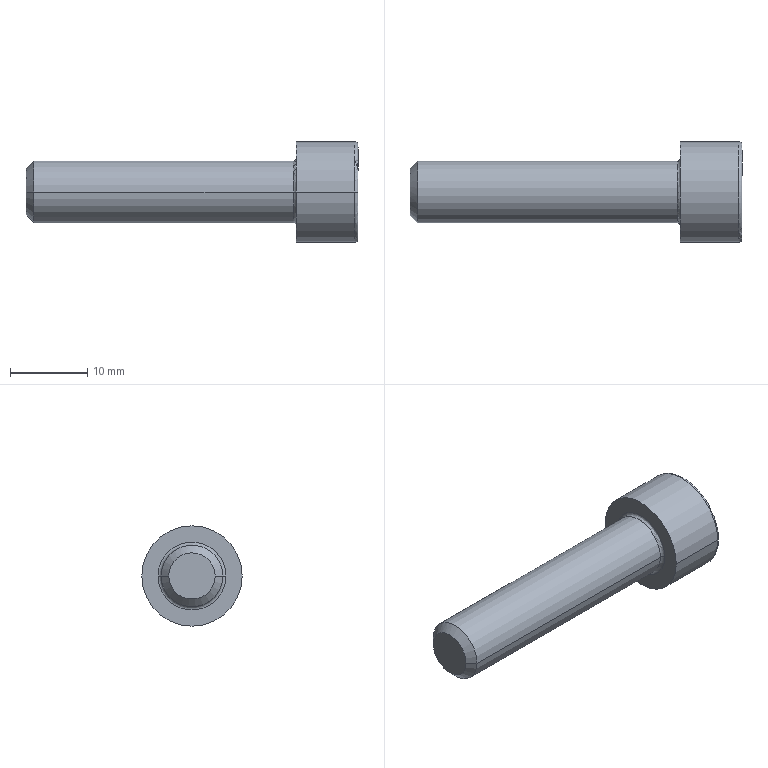Part | STEP file | Positioning_id2042_x_t | 1 solid | 20 faces | box 43 x 13 x 13 mm | volume 2687 mm3 | plane 10 | torus 4 | cylinder 4 | cone 2 | commonest cylinder face diameters 8 x2 13 x2
STEP:
#1=CARTESIAN_POINT('',(0.,0.,0.));
#2=DIRECTION('',(0.,0.,1.));
#3=DIRECTION('',(1.,0.,0.));
#4=AXIS2_PLACEMENT_3D('',#1,#2,#3);
#5=CARTESIAN_POINT('',(-1027.002,-38.,396.5));
#6=VERTEX_POINT('',#5);
#7=CARTESIAN_POINT('',(-1026.002,-39.,396.5));
#8=VERTEX_POINT('',#7);
#9=CARTESIAN_POINT('',(-1027.002,-38.,396.5));
#10=DIRECTION('',(0.7071,-0.7071,0.));
#11=VECTOR('',#10,1.);
#12=LINE('',#9,#11);
#13=CARTESIAN_POINT('',(-1026.002,-35.,396.5));
#14=DIRECTION('',(1.,0.,0.));
#15=DIRECTION('',(0.,-1.,0.));
#16=AXIS2_PLACEMENT_3D('',#13,#14,#15);
#17=CONICAL_SURFACE('',#16,4.,0.7854);
#18=CARTESIAN_POINT('',(0.,-1.));
#19=DIRECTION('',(0.,1.));
#20=VECTOR('',#19,1.);
#21=LINE('',#18,#20);
#22=(GEOMETRIC_REPRESENTATION_CONTEXT(2)PARAMETRIC_REPRESENTATION_CONTEXT()REPRESENTATION_CONTEXT('',''));
#23=DEFINITIONAL_REPRESENTATION('',(#21),#22);
#24=PCURVE('',#17,#23);
#25=CARTESIAN_POINT('',(-1026.002,-35.,396.5));
#26=DIRECTION('',(1.,0.,0.));
#27=DIRECTION('',(0.,-1.,0.));
#28=AXIS2_PLACEMENT_3D('',#25,#26,#27);
#29=CONICAL_SURFACE('',#28,4.,0.7854);
#30=CARTESIAN_POINT('',(6.283,-1.));
#31=DIRECTION('',(0.,1.));
#32=VECTOR('',#31,1.);
#33=LINE('',#30,#32);
#34=(GEOMETRIC_REPRESENTATION_CONTEXT(2)PARAMETRIC_REPRESENTATION_CONTEXT()REPRESENTATION_CONTEXT('',''));
#35=DEFINITIONAL_REPRESENTATION('',(#33),#34);
#36=PCURVE('',#29,#35);
#37=SURFACE_CURVE('',#12,(#24,#36),.PCURVE_S1.);
#38=EDGE_CURVE('',#6,#8,#37,.T.);
#39=ORIENTED_EDGE('',*,*,#38,.F.);
#40=CARTESIAN_POINT('',(-1027.002,-32.,396.5));
#41=VERTEX_POINT('',#40);
#42=CARTESIAN_POINT('',(-1027.002,-35.,396.5));
#43=DIRECTION('',(-1.,0.,0.));
#44=DIRECTION('',(0.,0.,-1.));
#45=AXIS2_PLACEMENT_3D('',#42,#43,#44);
#46=CIRCLE('',#45,3.);
#47=CARTESIAN_POINT('',(7.854,-1.));
#48=DIRECTION('',(-1.,0.));
#49=VECTOR('',#48,1.);
#50=LINE('',#47,#49);
#51=(GEOMETRIC_REPRESENTATION_CONTEXT(2)PARAMETRIC_REPRESENTATION_CONTEXT()REPRESENTATION_CONTEXT('',''));
#52=DEFINITIONAL_REPRESENTATION('',(#50),#51);
#53=PCURVE('',#17,#52);
#54=CARTESIAN_POINT('',(-1027.002,-35.,396.5));
#55=DIRECTION('',(-1.,0.,0.));
#56=DIRECTION('',(0.,0.,-1.));
#57=AXIS2_PLACEMENT_3D('',#54,#55,#56);
#58=PLANE('',#57);
#59=CARTESIAN_POINT('',(0.,0.));
#60=DIRECTION('',(1.,0.));
#61=AXIS2_PLACEMENT_2D('',#59,#60);
#62=CIRCLE('',#61,3.);
#63=(GEOMETRIC_REPRESENTATION_CONTEXT(2)PARAMETRIC_REPRESENTATION_CONTEXT()REPRESENTATION_CONTEXT('',''));
#64=DEFINITIONAL_REPRESENTATION('',(#62),#63);
#65=PCURVE('',#58,#64);
#66=SURFACE_CURVE('',#46,(#53,#65),.PCURVE_S1.);
#67=EDGE_CURVE('',#41,#6,#66,.T.);
#68=ORIENTED_EDGE('',*,*,#67,.F.);
#69=CARTESIAN_POINT('',(-1026.002,-31.,396.5));
#70=VERTEX_POINT('',#69);
#71=CARTESIAN_POINT('',(-1027.002,-32.,396.5));
#72=DIRECTION('',(-0.7071,-0.7071,0.));
#73=VECTOR('',#72,1.);
#74=LINE('',#71,#73);
#75=CARTESIAN_POINT('',(3.142,-1.));
#76=DIRECTION('',(0.,-1.));
#77=VECTOR('',#76,1.);
#78=LINE('',#75,#77);
#79=(GEOMETRIC_REPRESENTATION_CONTEXT(2)PARAMETRIC_REPRESENTATION_CONTEXT()REPRESENTATION_CONTEXT('',''));
#80=DEFINITIONAL_REPRESENTATION('',(#78),#79);
#81=PCURVE('',#17,#80);
#82=CARTESIAN_POINT('',(3.142,-1.));
#83=DIRECTION('',(0.,-1.));
#84=VECTOR('',#83,1.);
#85=LINE('',#82,#84);
#86=(GEOMETRIC_REPRESENTATION_CONTEXT(2)PARAMETRIC_REPRESENTATION_CONTEXT()REPRESENTATION_CONTEXT('',''));
#87=DEFINITIONAL_REPRESENTATION('',(#85),#86);
#88=PCURVE('',#29,#87);
#89=SURFACE_CURVE('',#74,(#81,#88),.PCURVE_S1.);
#90=EDGE_CURVE('',#70,#41,#89,.T.);
#91=ORIENTED_EDGE('',*,*,#90,.F.);
#92=CARTESIAN_POINT('',(-1026.002,-35.,396.5));
#93=DIRECTION('',(1.,0.,0.));
#94=DIRECTION('',(0.,-1.,0.));
#95=AXIS2_PLACEMENT_3D('',#92,#93,#94);
#96=CIRCLE('',#95,4.);
#97=CARTESIAN_POINT('',(0.,0.));
#98=DIRECTION('',(1.,0.));
#99=VECTOR('',#98,1.);
#100=LINE('',#97,#99);
#101=(GEOMETRIC_REPRESENTATION_CONTEXT(2)PARAMETRIC_REPRESENTATION_CONTEXT()REPRESENTATION_CONTEXT('',''));
#102=DEFINITIONAL_REPRESENTATION('',(#100),#101);
#103=PCURVE('',#17,#102);
#104=CARTESIAN_POINT('',(-992.002,-35.,396.5));
#105=DIRECTION('',(-1.,0.,0.));
#106=DIRECTION('',(0.,-1.,0.));
#107=AXIS2_PLACEMENT_3D('',#104,#105,#106);
#108=CYLINDRICAL_SURFACE('',#107,4.);
#109=CARTESIAN_POINT('',(6.283,34.));
#110=DIRECTION('',(-1.,0.));
#111=VECTOR('',#110,1.);
#112=LINE('',#109,#111);
#113=(GEOMETRIC_REPRESENTATION_CONTEXT(2)PARAMETRIC_REPRESENTATION_CONTEXT()REPRESENTATION_CONTEXT('',''));
#114=DEFINITIONAL_REPRESENTATION('',(#112),#113);
#115=PCURVE('',#108,#114);
#116=SURFACE_CURVE('',#96,(#103,#115),.PCURVE_S1.);
#117=EDGE_CURVE('',#8,#70,#116,.T.);
#118=ORIENTED_EDGE('',*,*,#117,.F.);
#119=EDGE_LOOP('',(#39,#68,#91,#118));
#120=FACE_BOUND('',#119,.T.);
#121=ADVANCED_FACE('',(#120),#17,.T.);
#122=CARTESIAN_POINT('',(-988.002,-35.,393.07));
#123=VERTEX_POINT('',#122);
#124=CARTESIAN_POINT('',(-988.002,-37.97,394.785));
#125=VERTEX_POINT('',#124);
#126=CARTESIAN_POINT('',(-988.002,-35.,393.07));
#127=DIRECTION('',(0.,-0.866,0.5));
#128=VECTOR('',#127,1.);
#129=LINE('',#126,#128);
#130=CARTESIAN_POINT('',(-988.002,-35.,393.07));
#131=DIRECTION('',(0.,0.5,0.866));
#132=DIRECTION('',(0.,-0.866,0.5));
#133=AXIS2_PLACEMENT_3D('',#130,#131,#132);
#134=PLANE('',#133);
#135=CARTESIAN_POINT('',(0.,0.));
#136=DIRECTION('',(1.,0.));
#137=VECTOR('',#136,1.);
#138=LINE('',#135,#137);
#139=(GEOMETRIC_REPRESENTATION_CONTEXT(2)PARAMETRIC_REPRESENTATION_CONTEXT()REPRESENTATION_CONTEXT('',''));
#140=DEFINITIONAL_REPRESENTATION('',(#138),#139);
#141=PCURVE('',#134,#140);
#142=CARTESIAN_POINT('',(-988.002,-37.97,398.215));
#143=DIRECTION('',(-1.,0.,0.));
#144=DIRECTION('',(0.,0.,-1.));
#145=AXIS2_PLACEMENT_3D('',#142,#143,#144);
#146=PLANE('',#145);
#147=CARTESIAN_POINT('',(5.145,-2.97));
#148=DIRECTION('',(-0.5,0.866));
#149=VECTOR('',#148,1.);
#150=LINE('',#147,#149);
#151=(GEOMETRIC_REPRESENTATION_CONTEXT(2)PARAMETRIC_REPRESENTATION_CONTEXT()REPRESENTATION_CONTEXT('',''));
#152=DEFINITIONAL_REPRESENTATION('',(#150),#151);
#153=PCURVE('',#146,#152);
#154=SURFACE_CURVE('',#129,(#141,#153),.PCURVE_S1.);
#155=EDGE_CURVE('',#123,#125,#154,.T.);
#156=ORIENTED_EDGE('',*,*,#155,.T.);
#157=CARTESIAN_POINT('',(-984.002,-37.97,394.785));
#158=VERTEX_POINT('',#157);
#159=CARTESIAN_POINT('',(-988.002,-37.97,394.785));
#160=DIRECTION('',(1.,0.,0.));
#161=VECTOR('',#160,1.);
#162=LINE('',#159,#161);
#163=CARTESIAN_POINT('',(3.43,0.));
#164=DIRECTION('',(0.,1.));
#165=VECTOR('',#164,1.);
#166=LINE('',#163,#165);
#167=(GEOMETRIC_REPRESENTATION_CONTEXT(2)PARAMETRIC_REPRESENTATION_CONTEXT()REPRESENTATION_CONTEXT('',''));
#168=DEFINITIONAL_REPRESENTATION('',(#166),#167);
#169=PCURVE('',#134,#168);
#170=CARTESIAN_POINT('',(-988.002,-37.97,394.785));
#171=DIRECTION('',(0.,1.,0.));
#172=DIRECTION('',(0.,0.,1.));
#173=AXIS2_PLACEMENT_3D('',#170,#171,#172);
#174=PLANE('',#173);
#175=CARTESIAN_POINT('',(0.,0.));
#176=DIRECTION('',(0.,1.));
#177=VECTOR('',#176,1.);
#178=LINE('',#175,#177);
#179=(GEOMETRIC_REPRESENTATION_CONTEXT(2)PARAMETRIC_REPRESENTATION_CONTEXT()REPRESENTATION_CONTEXT('',''));
#180=DEFINITIONAL_REPRESENTATION('',(#178),#179);
#181=PCURVE('',#174,#180);
#182=SURFACE_CURVE('',#162,(#169,#181),.PCURVE_S1.);
#183=EDGE_CURVE('',#125,#158,#182,.T.);
#184=ORIENTED_EDGE('',*,*,#183,.T.);
#185=CARTESIAN_POINT('',(-984.002,-35.,393.07));
#186=VERTEX_POINT('',#185);
#187=CARTESIAN_POINT('',(-984.002,-35.,393.07));
#188=DIRECTION('',(0.,-0.866,0.5));
#189=VECTOR('',#188,1.);
#190=LINE('',#187,#189);
#191=CARTESIAN_POINT('',(0.,4.));
#192=DIRECTION('',(1.,0.));
#193=VECTOR('',#192,1.);
#194=LINE('',#191,#193);
#195=(GEOMETRIC_REPRESENTATION_CONTEXT(2)PARAMETRIC_REPRESENTATION_CONTEXT()REPRESENTATION_CONTEXT('',''));
#196=DEFINITIONAL_REPRESENTATION('',(#194),#195);
#197=PCURVE('',#134,#196);
#198=CARTESIAN_POINT('',(-984.002,-35.,396.5));
#199=DIRECTION('',(1.,0.,0.));
#200=DIRECTION('',(0.,-1.,0.));
#201=AXIS2_PLACEMENT_3D('',#198,#199,#200);
#202=PLANE('',#201);
#203=CARTESIAN_POINT('',(0.,3.43));
#204=DIRECTION('',(0.866,-0.5));
#205=VECTOR('',#204,1.);
#206=LINE('',#203,#205);
#207=(GEOMETRIC_REPRESENTATION_CONTEXT(2)PARAMETRIC_REPRESENTATION_CONTEXT()REPRESENTATION_CONTEXT('',''));
#208=DEFINITIONAL_REPRESENTATION('',(#206),#207);
#209=PCURVE('',#202,#208);
#210=SURFACE_CURVE('',#190,(#197,#209),.PCURVE_S1.);
#211=EDGE_CURVE('',#186,#158,#210,.T.);
#212=ORIENTED_EDGE('',*,*,#211,.F.);
#213=CARTESIAN_POINT('',(-988.002,-35.,393.07));
#214=DIRECTION('',(1.,0.,0.));
#215=VECTOR('',#214,1.);
#216=LINE('',#213,#215);
#217=CARTESIAN_POINT('',(0.,0.));
#218=DIRECTION('',(0.,1.));
#219=VECTOR('',#218,1.);
#220=LINE('',#217,#219);
#221=(GEOMETRIC_REPRESENTATION_CONTEXT(2)PARAMETRIC_REPRESENTATION_CONTEXT()REPRESENTATION_CONTEXT('',''));
#222=DEFINITIONAL_REPRESENTATION('',(#220),#221);
#223=PCURVE('',#134,#222);
#224=CARTESIAN_POINT('',(-988.002,-32.03,394.785));
#225=DIRECTION('',(0.,-0.5,0.866));
#226=DIRECTION('',(0.,-0.866,-0.5));
#227=AXIS2_PLACEMENT_3D('',#224,#225,#226);
#228=PLANE('',#227);
#229=CARTESIAN_POINT('',(3.43,0.));
#230=DIRECTION('',(0.,1.));
#231=VECTOR('',#230,1.);
#232=LINE('',#229,#231);
#233=(GEOMETRIC_REPRESENTATION_CONTEXT(2)PARAMETRIC_REPRESENTATION_CONTEXT()REPRESENTATION_CONTEXT('',''));
#234=DEFINITIONAL_REPRESENTATION('',(#232),#233);
#235=PCURVE('',#228,#234);
#236=SURFACE_CURVE('',#216,(#223,#235),.PCURVE_S1.);
#237=EDGE_CURVE('',#123,#186,#236,.T.);
#238=ORIENTED_EDGE('',*,*,#237,.F.);
#239=EDGE_LOOP('',(#156,#184,#212,#238));
#240=FACE_BOUND('',#239,.T.);
#241=ADVANCED_FACE('',(#240),#134,.T.);
#242=CARTESIAN_POINT('',(-988.002,-37.97,398.215));
#243=VERTEX_POINT('',#242);
#244=CARTESIAN_POINT('',(-988.002,-37.97,394.785));
#245=DIRECTION('',(0.,0.,1.));
#246=VECTOR('',#245,1.);
#247=LINE('',#244,#246);
#248=CARTESIAN_POINT('',(3.43,0.));
#249=DIRECTION('',(-1.,0.));
#250=VECTOR('',#249,1.);
#251=LINE('',#248,#250);
#252=(GEOMETRIC_REPRESENTATION_CONTEXT(2)PARAMETRIC_REPRESENTATION_CONTEXT()REPRESENTATION_CONTEXT('',''));
#253=DEFINITIONAL_REPRESENTATION('',(#251),#252);
#254=PCURVE('',#146,#253);
#255=CARTESIAN_POINT('',(0.,0.));
#256=DIRECTION('',(1.,0.));
#257=VECTOR('',#256,1.);
#258=LINE('',#255,#257);
#259=(GEOMETRIC_REPRESENTATION_CONTEXT(2)PARAMETRIC_REPRESENTATION_CONTEXT()REPRESENTATION_CONTEXT('',''));
#260=DEFINITIONAL_REPRESENTATION('',(#258),#259);
#261=PCURVE('',#174,#260);
#262=SURFACE_CURVE('',#247,(#254,#261),.PCURVE_S1.);
#263=EDGE_CURVE('',#125,#243,#262,.T.);
#264=ORIENTED_EDGE('',*,*,#263,.F.);
#265=ORIENTED_EDGE('',*,*,#155,.F.);
#266=CARTESIAN_POINT('',(-988.002,-32.03,394.785));
#267=VERTEX_POINT('',#266);
#268=CARTESIAN_POINT('',(-988.002,-32.03,394.785));
#269=DIRECTION('',(0.,-0.866,-0.5));
#270=VECTOR('',#269,1.);
#271=LINE('',#268,#270);
#272=CARTESIAN_POINT('',(3.43,-5.941));
#273=DIRECTION('',(0.5,0.866));
#274=VECTOR('',#273,1.);
#275=LINE('',#272,#274);
#276=(GEOMETRIC_REPRESENTATION_CONTEXT(2)PARAMETRIC_REPRESENTATION_CONTEXT()REPRESENTATION_CONTEXT('',''));
#277=DEFINITIONAL_REPRESENTATION('',(#275),#276);
#278=PCURVE('',#146,#277);
#279=CARTESIAN_POINT('',(0.,0.));
#280=DIRECTION('',(1.,0.));
#281=VECTOR('',#280,1.);
#282=LINE('',#279,#281);
#283=(GEOMETRIC_REPRESENTATION_CONTEXT(2)PARAMETRIC_REPRESENTATION_CONTEXT()REPRESENTATION_CONTEXT('',''));
#284=DEFINITIONAL_REPRESENTATION('',(#282),#283);
#285=PCURVE('',#228,#284);
#286=SURFACE_CURVE('',#271,(#278,#285),.PCURVE_S1.);
#287=EDGE_CURVE('',#267,#123,#286,.T.);
#288=ORIENTED_EDGE('',*,*,#287,.F.);
#289=CARTESIAN_POINT('',(-988.002,-32.03,398.215));
#290=VERTEX_POINT('',#289);
#291=CARTESIAN_POINT('',(-988.002,-32.03,398.215));
#292=DIRECTION('',(0.,0.,-1.));
#293=VECTOR('',#292,1.);
#294=LINE('',#291,#293);
#295=CARTESIAN_POINT('',(0.,-5.941));
#296=DIRECTION('',(1.,0.));
#297=VECTOR('',#296,1.);
#298=LINE('',#295,#297);
#299=(GEOMETRIC_REPRESENTATION_CONTEXT(2)PARAMETRIC_REPRESENTATION_CONTEXT()REPRESENTATION_CONTEXT('',''));
#300=DEFINITIONAL_REPRESENTATION('',(#298),#299);
#301=PCURVE('',#146,#300);
#302=CARTESIAN_POINT('',(-988.002,-32.03,398.215));
#303=DIRECTION('',(0.,-1.,0.));
#304=DIRECTION('',(0.,0.,-1.));
#305=AXIS2_PLACEMENT_3D('',#302,#303,#304);
#306=PLANE('',#305);
#307=CARTESIAN_POINT('',(0.,0.));
#308=DIRECTION('',(1.,0.));
#309=VECTOR('',#308,1.);
#310=LINE('',#307,#309);
#311=(GEOMETRIC_REPRESENTATION_CONTEXT(2)PARAMETRIC_REPRESENTATION_CONTEXT()REPRESENTATION_CONTEXT('',''));
#312=DEFINITIONAL_REPRESENTATION('',(#310),#311);
#313=PCURVE('',#306,#312);
#314=SURFACE_CURVE('',#294,(#301,#313),.PCURVE_S1.);
#315=EDGE_CURVE('',#290,#267,#314,.T.);
#316=ORIENTED_EDGE('',*,*,#315,.F.);
#317=CARTESIAN_POINT('',(-988.002,-35.,399.93));
#318=VERTEX_POINT('',#317);
#319=CARTESIAN_POINT('',(-988.002,-35.,399.93));
#320=DIRECTION('',(0.,0.866,-0.5));
#321=VECTOR('',#320,1.);
#322=LINE('',#319,#321);
#323=CARTESIAN_POINT('',(-1.715,-2.97));
#324=DIRECTION('',(0.5,-0.866));
#325=VECTOR('',#324,1.);
#326=LINE('',#323,#325);
#327=(GEOMETRIC_REPRESENTATION_CONTEXT(2)PARAMETRIC_REPRESENTATION_CONTEXT()REPRESENTATION_CONTEXT('',''));
#328=DEFINITIONAL_REPRESENTATION('',(#326),#327);
#329=PCURVE('',#146,#328);
#330=CARTESIAN_POINT('',(-988.002,-35.,399.93));
#331=DIRECTION('',(0.,-0.5,-0.866));
#332=DIRECTION('',(0.,0.866,-0.5));
#333=AXIS2_PLACEMENT_3D('',#330,#331,#332);
#334=PLANE('',#333);
#335=CARTESIAN_POINT('',(0.,0.));
#336=DIRECTION('',(1.,0.));
#337=VECTOR('',#336,1.);
#338=LINE('',#335,#337);
#339=(GEOMETRIC_REPRESENTATION_CONTEXT(2)PARAMETRIC_REPRESENTATION_CONTEXT()REPRESENTATION_CONTEXT('',''));
#340=DEFINITIONAL_REPRESENTATION('',(#338),#339);
#341=PCURVE('',#334,#340);
#342=SURFACE_CURVE('',#322,(#329,#341),.PCURVE_S1.);
#343=EDGE_CURVE('',#318,#290,#342,.T.);
#344=ORIENTED_EDGE('',*,*,#343,.F.);
#345=CARTESIAN_POINT('',(-988.002,-37.97,398.215));
#346=DIRECTION('',(0.,0.866,0.5));
#347=VECTOR('',#346,1.);
#348=LINE('',#345,#347);
#349=CARTESIAN_POINT('',(0.,0.));
#350=DIRECTION('',(-0.5,-0.866));
#351=VECTOR('',#350,1.);
#352=LINE('',#349,#351);
#353=(GEOMETRIC_REPRESENTATION_CONTEXT(2)PARAMETRIC_REPRESENTATION_CONTEXT()REPRESENTATION_CONTEXT('',''));
#354=DEFINITIONAL_REPRESENTATION('',(#352),#353);
#355=PCURVE('',#146,#354);
#356=CARTESIAN_POINT('',(-988.002,-37.97,398.215));
#357=DIRECTION('',(0.,0.5,-0.866));
#358=DIRECTION('',(0.,0.866,0.5));
#359=AXIS2_PLACEMENT_3D('',#356,#357,#358);
#360=PLANE('',#359);
#361=CARTESIAN_POINT('',(0.,0.));
#362=DIRECTION('',(1.,0.));
#363=VECTOR('',#362,1.);
#364=LINE('',#361,#363);
#365=(GEOMETRIC_REPRESENTATION_CONTEXT(2)PARAMETRIC_REPRESENTATION_CONTEXT()REPRESENTATION_CONTEXT('',''));
#366=DEFINITIONAL_REPRESENTATION('',(#364),#365);
#367=PCURVE('',#360,#366);
#368=SURFACE_CURVE('',#348,(#355,#367),.PCURVE_S1.);
#369=EDGE_CURVE('',#243,#318,#368,.T.);
#370=ORIENTED_EDGE('',*,*,#369,.F.);
#371=EDGE_LOOP('',(#264,#265,#288,#316,#344,#370));
#372=FACE_BOUND('',#371,.T.);
#373=ADVANCED_FACE('',(#372),#146,.F.);
#374=ORIENTED_EDGE('',*,*,#237,.T.);
#375=CARTESIAN_POINT('',(-984.002,-32.03,394.785));
#376=VERTEX_POINT('',#375);
#377=CARTESIAN_POINT('',(-984.002,-32.03,394.785));
#378=DIRECTION('',(0.,-0.866,-0.5));
#379=VECTOR('',#378,1.);
#380=LINE('',#377,#379);
#381=CARTESIAN_POINT('',(0.,4.));
#382=DIRECTION('',(1.,0.));
#383=VECTOR('',#382,1.);
#384=LINE('',#381,#383);
#385=(GEOMETRIC_REPRESENTATION_CONTEXT(2)PARAMETRIC_REPRESENTATION_CONTEXT()REPRESENTATION_CONTEXT('',''));
#386=DEFINITIONAL_REPRESENTATION('',(#384),#385);
#387=PCURVE('',#228,#386);
#388=CARTESIAN_POINT('',(-2.97,1.715));
#389=DIRECTION('',(0.866,0.5));
#390=VECTOR('',#389,1.);
#391=LINE('',#388,#390);
#392=(GEOMETRIC_REPRESENTATION_CONTEXT(2)PARAMETRIC_REPRESENTATION_CONTEXT()REPRESENTATION_CONTEXT('',''));
#393=DEFINITIONAL_REPRESENTATION('',(#391),#392);
#394=PCURVE('',#202,#393);
#395=SURFACE_CURVE('',#380,(#387,#394),.PCURVE_S1.);
#396=EDGE_CURVE('',#376,#186,#395,.T.);
#397=ORIENTED_EDGE('',*,*,#396,.F.);
#398=CARTESIAN_POINT('',(-988.002,-32.03,394.785));
#399=DIRECTION('',(1.,0.,0.));
#400=VECTOR('',#399,1.);
#401=LINE('',#398,#400);
#402=CARTESIAN_POINT('',(0.,0.));
#403=DIRECTION('',(0.,1.));
#404=VECTOR('',#403,1.);
#405=LINE('',#402,#404);
#406=(GEOMETRIC_REPRESENTATION_CONTEXT(2)PARAMETRIC_REPRESENTATION_CONTEXT()REPRESENTATION_CONTEXT('',''));
#407=DEFINITIONAL_REPRESENTATION('',(#405),#406);
#408=PCURVE('',#228,#407);
#409=CARTESIAN_POINT('',(3.43,0.));
#410=DIRECTION('',(0.,1.));
#411=VECTOR('',#410,1.);
#412=LINE('',#409,#411);
#413=(GEOMETRIC_REPRESENTATION_CONTEXT(2)PARAMETRIC_REPRESENTATION_CONTEXT()REPRESENTATION_CONTEXT('',''));
#414=DEFINITIONAL_REPRESENTATION('',(#412),#413);
#415=PCURVE('',#306,#414);
#416=SURFACE_CURVE('',#401,(#408,#415),.PCURVE_S1.);
#417=EDGE_CURVE('',#267,#376,#416,.T.);
#418=ORIENTED_EDGE('',*,*,#417,.F.);
#419=ORIENTED_EDGE('',*,*,#287,.T.);
#420=EDGE_LOOP('',(#374,#397,#418,#419));
#421=FACE_BOUND('',#420,.T.);
#422=ADVANCED_FACE('',(#421),#228,.T.);
#423=ORIENTED_EDGE('',*,*,#417,.T.);
#424=CARTESIAN_POINT('',(-984.002,-32.03,398.215));
#425=VERTEX_POINT('',#424);
#426=CARTESIAN_POINT('',(-984.002,-32.03,398.215));
#427=DIRECTION('',(0.,0.,-1.));
#428=VECTOR('',#427,1.);
#429=LINE('',#426,#428);
#430=CARTESIAN_POINT('',(0.,4.));
#431=DIRECTION('',(1.,0.));
#432=VECTOR('',#431,1.);
#433=LINE('',#430,#432);
#434=(GEOMETRIC_REPRESENTATION_CONTEXT(2)PARAMETRIC_REPRESENTATION_CONTEXT()REPRESENTATION_CONTEXT('',''));
#435=DEFINITIONAL_REPRESENTATION('',(#433),#434);
#436=PCURVE('',#306,#435);
#437=CARTESIAN_POINT('',(-2.97,-1.715));
#438=DIRECTION('',(0.,1.));
#439=VECTOR('',#438,1.);
#440=LINE('',#437,#439);
#441=(GEOMETRIC_REPRESENTATION_CONTEXT(2)PARAMETRIC_REPRESENTATION_CONTEXT()REPRESENTATION_CONTEXT('',''));
#442=DEFINITIONAL_REPRESENTATION('',(#440),#441);
#443=PCURVE('',#202,#442);
#444=SURFACE_CURVE('',#429,(#436,#443),.PCURVE_S1.);
#445=EDGE_CURVE('',#425,#376,#444,.T.);
#446=ORIENTED_EDGE('',*,*,#445,.F.);
#447=CARTESIAN_POINT('',(-988.002,-32.03,398.215));
#448=DIRECTION('',(1.,0.,0.));
#449=VECTOR('',#448,1.);
#450=LINE('',#447,#449);
#451=CARTESIAN_POINT('',(0.,0.));
#452=DIRECTION('',(0.,1.));
#453=VECTOR('',#452,1.);
#454=LINE('',#451,#453);
#455=(GEOMETRIC_REPRESENTATION_CONTEXT(2)PARAMETRIC_REPRESENTATION_CONTEXT()REPRESENTATION_CONTEXT('',''));
#456=DEFINITIONAL_REPRESENTATION('',(#454),#455);
#457=PCURVE('',#306,#456);
#458=CARTESIAN_POINT('',(3.43,0.));
#459=DIRECTION('',(0.,1.));
#460=VECTOR('',#459,1.);
#461=LINE('',#458,#460);
#462=(GEOMETRIC_REPRESENTATION_CONTEXT(2)PARAMETRIC_REPRESENTATION_CONTEXT()REPRESENTATION_CONTEXT('',''));
#463=DEFINITIONAL_REPRESENTATION('',(#461),#462);
#464=PCURVE('',#334,#463);
#465=SURFACE_CURVE('',#450,(#457,#464),.PCURVE_S1.);
#466=EDGE_CURVE('',#290,#425,#465,.T.);
#467=ORIENTED_EDGE('',*,*,#466,.F.);
#468=ORIENTED_EDGE('',*,*,#315,.T.);
#469=EDGE_LOOP('',(#423,#446,#467,#468));
#470=FACE_BOUND('',#469,.T.);
#471=ADVANCED_FACE('',(#470),#306,.T.);
#472=ORIENTED_EDGE('',*,*,#466,.T.);
#473=CARTESIAN_POINT('',(-984.002,-35.,399.93));
#474=VERTEX_POINT('',#473);
#475=CARTESIAN_POINT('',(-984.002,-35.,399.93));
#476=DIRECTION('',(0.,0.866,-0.5));
#477=VECTOR('',#476,1.);
#478=LINE('',#475,#477);
#479=CARTESIAN_POINT('',(0.,4.));
#480=DIRECTION('',(1.,0.));
#481=VECTOR('',#480,1.);
#482=LINE('',#479,#481);
#483=(GEOMETRIC_REPRESENTATION_CONTEXT(2)PARAMETRIC_REPRESENTATION_CONTEXT()REPRESENTATION_CONTEXT('',''));
#484=DEFINITIONAL_REPRESENTATION('',(#482),#483);
#485=PCURVE('',#334,#484);
#486=CARTESIAN_POINT('',(0.,-3.43));
#487=DIRECTION('',(-0.866,0.5));
#488=VECTOR('',#487,1.);
#489=LINE('',#486,#488);
#490=(GEOMETRIC_REPRESENTATION_CONTEXT(2)PARAMETRIC_REPRESENTATION_CONTEXT()REPRESENTATION_CONTEXT('',''));
#491=DEFINITIONAL_REPRESENTATION('',(#489),#490);
#492=PCURVE('',#202,#491);
#493=SURFACE_CURVE('',#478,(#485,#492),.PCURVE_S1.);
#494=EDGE_CURVE('',#474,#425,#493,.T.);
#495=ORIENTED_EDGE('',*,*,#494,.F.);
#496=CARTESIAN_POINT('',(-988.002,-35.,399.93));
#497=DIRECTION('',(1.,0.,0.));
#498=VECTOR('',#497,1.);
#499=LINE('',#496,#498);
#500=CARTESIAN_POINT('',(0.,0.));
#501=DIRECTION('',(0.,1.));
#502=VECTOR('',#501,1.);
#503=LINE('',#500,#502);
#504=(GEOMETRIC_REPRESENTATION_CONTEXT(2)PARAMETRIC_REPRESENTATION_CONTEXT()REPRESENTATION_CONTEXT('',''));
#505=DEFINITIONAL_REPRESENTATION('',(#503),#504);
#506=PCURVE('',#334,#505);
#507=CARTESIAN_POINT('',(3.43,0.));
#508=DIRECTION('',(0.,1.));
#509=VECTOR('',#508,1.);
#510=LINE('',#507,#509);
#511=(GEOMETRIC_REPRESENTATION_CONTEXT(2)PARAMETRIC_REPRESENTATION_CONTEXT()REPRESENTATION_CONTEXT('',''));
#512=DEFINITIONAL_REPRESENTATION('',(#510),#511);
#513=PCURVE('',#360,#512);
#514=SURFACE_CURVE('',#499,(#506,#513),.PCURVE_S1.);
#515=EDGE_CURVE('',#318,#474,#514,.T.);
#516=ORIENTED_EDGE('',*,*,#515,.F.);
#517=ORIENTED_EDGE('',*,*,#343,.T.);
#518=EDGE_LOOP('',(#472,#495,#516,#517));
#519=FACE_BOUND('',#518,.T.);
#520=ADVANCED_FACE('',(#519),#334,.T.);
#521=ORIENTED_EDGE('',*,*,#515,.T.);
#522=CARTESIAN_POINT('',(-984.002,-37.97,398.215));
#523=VERTEX_POINT('',#522);
#524=CARTESIAN_POINT('',(-984.002,-37.97,398.215));
#525=DIRECTION('',(0.,0.866,0.5));
#526=VECTOR('',#525,1.);
#527=LINE('',#524,#526);
#528=CARTESIAN_POINT('',(0.,4.));
#529=DIRECTION('',(1.,0.));
#530=VECTOR('',#529,1.);
#531=LINE('',#528,#530);
#532=(GEOMETRIC_REPRESENTATION_CONTEXT(2)PARAMETRIC_REPRESENTATION_CONTEXT()REPRESENTATION_CONTEXT('',''));
#533=DEFINITIONAL_REPRESENTATION('',(#531),#532);
#534=PCURVE('',#360,#533);
#535=CARTESIAN_POINT('',(2.97,-1.715));
#536=DIRECTION('',(-0.866,-0.5));
#537=VECTOR('',#536,1.);
#538=LINE('',#535,#537);
#539=(GEOMETRIC_REPRESENTATION_CONTEXT(2)PARAMETRIC_REPRESENTATION_CONTEXT()REPRESENTATION_CONTEXT('',''));
#540=DEFINITIONAL_REPRESENTATION('',(#538),#539);
#541=PCURVE('',#202,#540);
#542=SURFACE_CURVE('',#527,(#534,#541),.PCURVE_S1.);
#543=EDGE_CURVE('',#523,#474,#542,.T.);
#544=ORIENTED_EDGE('',*,*,#543,.F.);
#545=CARTESIAN_POINT('',(-988.002,-37.97,398.215));
#546=DIRECTION('',(1.,0.,0.));
#547=VECTOR('',#546,1.);
#548=LINE('',#545,#547);
#549=CARTESIAN_POINT('',(0.,0.));
#550=DIRECTION('',(0.,1.));
#551=VECTOR('',#550,1.);
#552=LINE('',#549,#551);
#553=(GEOMETRIC_REPRESENTATION_CONTEXT(2)PARAMETRIC_REPRESENTATION_CONTEXT()REPRESENTATION_CONTEXT('',''));
#554=DEFINITIONAL_REPRESENTATION('',(#552),#553);
#555=PCURVE('',#360,#554);
#556=CARTESIAN_POINT('',(3.43,0.));
#557=DIRECTION('',(0.,1.));
#558=VECTOR('',#557,1.);
#559=LINE('',#556,#558);
#560=(GEOMETRIC_REPRESENTATION_CONTEXT(2)PARAMETRIC_REPRESENTATION_CONTEXT()REPRESENTATION_CONTEXT('',''));
#561=DEFINITIONAL_REPRESENTATION('',(#559),#560);
#562=PCURVE('',#174,#561);
#563=SURFACE_CURVE('',#548,(#555,#562),.PCURVE_S1.);
#564=EDGE_CURVE('',#243,#523,#563,.T.);
#565=ORIENTED_EDGE('',*,*,#564,.F.);
#566=ORIENTED_EDGE('',*,*,#369,.T.);
#567=EDGE_LOOP('',(#521,#544,#565,#566));
#568=FACE_BOUND('',#567,.T.);
#569=ADVANCED_FACE('',(#568),#360,.T.);
#570=ORIENTED_EDGE('',*,*,#564,.T.);
#571=CARTESIAN_POINT('',(-984.002,-37.97,394.785));
#572=DIRECTION('',(0.,0.,1.));
#573=VECTOR('',#572,1.);
#574=LINE('',#571,#573);
#575=CARTESIAN_POINT('',(0.,4.));
#576=DIRECTION('',(1.,0.));
#577=VECTOR('',#576,1.);
#578=LINE('',#575,#577);
#579=(GEOMETRIC_REPRESENTATION_CONTEXT(2)PARAMETRIC_REPRESENTATION_CONTEXT()REPRESENTATION_CONTEXT('',''));
#580=DEFINITIONAL_REPRESENTATION('',(#578),#579);
#581=PCURVE('',#174,#580);
#582=CARTESIAN_POINT('',(2.97,1.715));
#583=DIRECTION('',(0.,-1.));
#584=VECTOR('',#583,1.);
#585=LINE('',#582,#584);
#586=(GEOMETRIC_REPRESENTATION_CONTEXT(2)PARAMETRIC_REPRESENTATION_CONTEXT()REPRESENTATION_CONTEXT('',''));
#587=DEFINITIONAL_REPRESENTATION('',(#585),#586);
#588=PCURVE('',#202,#587);
#589=SURFACE_CURVE('',#574,(#581,#588),.PCURVE_S1.);
#590=EDGE_CURVE('',#158,#523,#589,.T.);
#591=ORIENTED_EDGE('',*,*,#590,.F.);
#592=ORIENTED_EDGE('',*,*,#183,.F.);
#593=ORIENTED_EDGE('',*,*,#263,.T.);
#594=EDGE_LOOP('',(#570,#591,#592,#593));
#595=FACE_BOUND('',#594,.T.);
#596=ADVANCED_FACE('',(#595),#174,.T.);
#597=CARTESIAN_POINT('',(-992.402,-31.,396.5));
#598=VERTEX_POINT('',#597);
#599=CARTESIAN_POINT('',(-992.402,-39.,396.5));
#600=VERTEX_POINT('',#599);
#601=CARTESIAN_POINT('',(-992.402,-35.,396.5));
#602=DIRECTION('',(1.,0.,0.));
#603=DIRECTION('',(0.,1.,0.));
#604=AXIS2_PLACEMENT_3D('',#601,#602,#603);
#605=CIRCLE('',#604,4.);
#606=CARTESIAN_POINT('',(-992.402,-35.,396.5));
#607=DIRECTION('',(1.,0.,0.));
#608=DIRECTION('',(0.,-1.,0.));
#609=AXIS2_PLACEMENT_3D('',#606,#607,#608);
#610=TOROIDAL_SURFACE('',#609,4.4,0.4);
#611=CARTESIAN_POINT('',(3.142,3.142));
#612=DIRECTION('',(1.,0.));
#613=VECTOR('',#612,1.);
#614=LINE('',#611,#613);
#615=(GEOMETRIC_REPRESENTATION_CONTEXT(2)PARAMETRIC_REPRESENTATION_CONTEXT()REPRESENTATION_CONTEXT('',''));
#616=DEFINITIONAL_REPRESENTATION('',(#614),#615);
#617=PCURVE('',#610,#616);
#618=CARTESIAN_POINT('',(-992.002,-35.,396.5));
#619=DIRECTION('',(-1.,0.,0.));
#620=DIRECTION('',(0.,-1.,0.));
#621=AXIS2_PLACEMENT_3D('',#618,#619,#620);
#622=CYLINDRICAL_SURFACE('',#621,4.);
#623=CARTESIAN_POINT('',(3.142,0.4));
#624=DIRECTION('',(-1.,0.));
#625=VECTOR('',#624,1.);
#626=LINE('',#623,#625);
#627=(GEOMETRIC_REPRESENTATION_CONTEXT(2)PARAMETRIC_REPRESENTATION_CONTEXT()REPRESENTATION_CONTEXT('',''));
#628=DEFINITIONAL_REPRESENTATION('',(#626),#627);
#629=PCURVE('',#622,#628);
#630=SURFACE_CURVE('',#605,(#617,#629),.PCURVE_S1.);
#631=EDGE_CURVE('',#598,#600,#630,.T.);
#632=ORIENTED_EDGE('',*,*,#631,.F.);
#633=CARTESIAN_POINT('',(-992.002,-30.6,396.5));
#634=VERTEX_POINT('',#633);
#635=CARTESIAN_POINT('',(-992.402,-30.6,396.5));
#636=DIRECTION('',(0.,0.,-1.));
#637=DIRECTION('',(1.,0.,0.));
#638=AXIS2_PLACEMENT_3D('',#635,#636,#637);
#639=CIRCLE('',#638,0.4);
#640=CARTESIAN_POINT('',(3.142,1.571));
#641=DIRECTION('',(0.,1.));
#642=VECTOR('',#641,1.);
#643=LINE('',#640,#642);
#644=(GEOMETRIC_REPRESENTATION_CONTEXT(2)PARAMETRIC_REPRESENTATION_CONTEXT()REPRESENTATION_CONTEXT('',''));
#645=DEFINITIONAL_REPRESENTATION('',(#643),#644);
#646=PCURVE('',#610,#645);
#647=CARTESIAN_POINT('',(-992.402,-35.,396.5));
#648=DIRECTION('',(1.,0.,0.));
#649=DIRECTION('',(0.,-1.,0.));
#650=AXIS2_PLACEMENT_3D('',#647,#648,#649);
#651=TOROIDAL_SURFACE('',#650,4.4,0.4);
#652=CARTESIAN_POINT('',(3.142,1.571));
#653=DIRECTION('',(0.,1.));
#654=VECTOR('',#653,1.);
#655=LINE('',#652,#654);
#656=(GEOMETRIC_REPRESENTATION_CONTEXT(2)PARAMETRIC_REPRESENTATION_CONTEXT()REPRESENTATION_CONTEXT('',''));
#657=DEFINITIONAL_REPRESENTATION('',(#655),#656);
#658=PCURVE('',#651,#657);
#659=SURFACE_CURVE('',#639,(#646,#658),.PCURVE_S1.);
#660=EDGE_CURVE('',#634,#598,#659,.T.);
#661=ORIENTED_EDGE('',*,*,#660,.F.);
#662=CARTESIAN_POINT('',(-992.002,-39.4,396.5));
#663=VERTEX_POINT('',#662);
#664=CARTESIAN_POINT('',(-992.002,-30.6,396.5));
#665=CARTESIAN_POINT('',(-992.002,-30.6,397.052));
#666=CARTESIAN_POINT('',(-992.002,-30.819,398.204));
#667=CARTESIAN_POINT('',(-992.002,-31.774,399.658));
#668=CARTESIAN_POINT('',(-992.002,-33.248,400.661));
#669=CARTESIAN_POINT('',(-992.002,-34.952,401.015));
#670=CARTESIAN_POINT('',(-992.002,-36.704,400.681));
#671=CARTESIAN_POINT('',(-992.002,-38.158,399.726));
#672=CARTESIAN_POINT('',(-992.002,-39.161,398.251));
#673=CARTESIAN_POINT('',(-992.002,-39.4,397.1));
#674=CARTESIAN_POINT('',(-992.002,-39.4,396.5));
#675=B_SPLINE_CURVE_WITH_KNOTS('',3,(#664,#665,#666,#667,#668,#669,#670,#671,#672,#673,#674),.UNSPECIFIED.,.F.,.F.,(4,1,1,1,1,1,1,1,4),(0.,0.1198,0.25,0.3698,0.5,0.6198,0.75,0.8698,1.),.UNSPECIFIED.);
#676=CARTESIAN_POINT('',(3.142,1.571));
#677=CARTESIAN_POINT('',(3.165,1.571));
#678=CARTESIAN_POINT('',(3.213,1.571));
#679=CARTESIAN_POINT('',(3.284,1.571));
#680=CARTESIAN_POINT('',(3.356,1.571));
#681=CARTESIAN_POINT('',(3.427,1.571));
#682=CARTESIAN_POINT('',(3.499,1.57));
#683=CARTESIAN_POINT('',(3.57,1.57));
#684=CARTESIAN_POINT('',(3.641,1.571));
#685=CARTESIAN_POINT('',(3.713,1.571));
#686=CARTESIAN_POINT('',(3.784,1.571));
#687=CARTESIAN_POINT('',(3.856,1.571));
#688=CARTESIAN_POINT('',(3.927,1.57));
#689=CARTESIAN_POINT('',(3.998,1.571));
#690=CARTESIAN_POINT('',(4.07,1.571));
#691=CARTESIAN_POINT('',(4.141,1.571));
#692=CARTESIAN_POINT('',(4.213,1.571));
#693=CARTESIAN_POINT('',(4.284,1.57));
#694=CARTESIAN_POINT('',(4.355,1.571));
#695=CARTESIAN_POINT('',(4.427,1.571));
#696=CARTESIAN_POINT('',(4.498,1.571));
#697=CARTESIAN_POINT('',(4.57,1.571));
#698=CARTESIAN_POINT('',(4.641,1.571));
#699=CARTESIAN_POINT('',(4.712,1.57));
#700=CARTESIAN_POINT('',(4.784,1.571));
#701=CARTESIAN_POINT('',(4.855,1.571));
#702=CARTESIAN_POINT('',(4.927,1.571));
#703=CARTESIAN_POINT('',(4.998,1.571));
#704=CARTESIAN_POINT('',(5.069,1.57));
#705=CARTESIAN_POINT('',(5.141,1.571));
#706=CARTESIAN_POINT('',(5.212,1.571));
#707=CARTESIAN_POINT('',(5.284,1.571));
#708=CARTESIAN_POINT('',(5.355,1.571));
#709=CARTESIAN_POINT('',(5.426,1.571));
#710=CARTESIAN_POINT('',(5.498,1.57));
#711=CARTESIAN_POINT('',(5.569,1.571));
#712=CARTESIAN_POINT('',(5.641,1.571));
#713=CARTESIAN_POINT('',(5.712,1.571));
#714=CARTESIAN_POINT('',(5.783,1.571));
#715=CARTESIAN_POINT('',(5.855,1.57));
#716=CARTESIAN_POINT('',(5.926,1.571));
#717=CARTESIAN_POINT('',(5.998,1.571));
#718=CARTESIAN_POINT('',(6.069,1.572));
#719=CARTESIAN_POINT('',(6.14,1.571));
#720=CARTESIAN_POINT('',(6.212,1.571));
#721=CARTESIAN_POINT('',(6.259,1.571));
#722=CARTESIAN_POINT('',(6.283,1.571));
#723=B_SPLINE_CURVE_WITH_KNOTS('',3,(#676,#677,#678,#679,#680,#681,#682,#683,#684,#685,#686,#687,#688,#689,#690,#691,#692,#693,#694,#695,#696,#697,#698,#699,#700,#701,#702,#703,#704,#705,#706,#707,#708,#709,#710,#711,#712,#713,#714,#715,#716,#717,#718,#719,#720,#721,#722),.UNSPECIFIED.,.F.,.F.,(4,1,1,1,1,1,1,1,1,1,1,1,1,1,1,1,1,1,1,1,1,1,1,1,1,1,1,1,1,1,1,1,1,1,1,1,1,1,1,1,1,1,1,1,4),(0.,0.02273,0.04545,0.06818,0.09091,0.1136,0.1364,0.1591,0.1818,0.2045,0.2273,0.25,0.2727,0.2955,0.3182,0.3409,0.3636,0.3864,0.4091,0.4318,0.4545,0.4773,0.5,0.5227,0.5455,0.5682,0.5909,0.6136,0.6364,0.6591,0.6818,0.7045,0.7273,0.75,0.7727,0.7955,0.8182,0.8409,0.8636,0.8864,0.9091,0.9318,0.9545,0.9773,1.),.QUASI_UNIFORM_KNOTS.);
#724=(GEOMETRIC_REPRESENTATION_CONTEXT(2)PARAMETRIC_REPRESENTATION_CONTEXT()REPRESENTATION_CONTEXT('',''));
#725=DEFINITIONAL_REPRESENTATION('',(#723),#724);
#726=PCURVE('',#610,#725);
#727=CARTESIAN_POINT('',(-992.002,-35.,403.));
#728=DIRECTION('',(-1.,0.,0.));
#729=DIRECTION('',(0.,1.,0.));
#730=AXIS2_PLACEMENT_3D('',#727,#728,#729);
#731=PLANE('',#730);
#732=CARTESIAN_POINT('',(4.4,6.5));
#733=CARTESIAN_POINT('',(4.4,5.948));
#734=CARTESIAN_POINT('',(4.181,4.796));
#735=CARTESIAN_POINT('',(3.226,3.342));
#736=CARTESIAN_POINT('',(1.752,2.339));
#737=CARTESIAN_POINT('',(0.04813,1.985));
#738=CARTESIAN_POINT('',(-1.704,2.319));
#739=CARTESIAN_POINT('',(-3.158,3.274));
#740=CARTESIAN_POINT('',(-4.161,4.749));
#741=CARTESIAN_POINT('',(-4.4,5.9));
#742=CARTESIAN_POINT('',(-4.4,6.5));
#743=B_SPLINE_CURVE_WITH_KNOTS('',3,(#732,#733,#734,#735,#736,#737,#738,#739,#740,#741,#742),.UNSPECIFIED.,.F.,.F.,(4,1,1,1,1,1,1,1,4),(0.,0.1198,0.25,0.3698,0.5,0.6198,0.75,0.8698,1.),.UNSPECIFIED.);
#744=(GEOMETRIC_REPRESENTATION_CONTEXT(2)PARAMETRIC_REPRESENTATION_CONTEXT()REPRESENTATION_CONTEXT('',''));
#745=DEFINITIONAL_REPRESENTATION('',(#743),#744);
#746=PCURVE('',#731,#745);
#747=SURFACE_CURVE('',#675,(#726,#746),.PCURVE_S1.);
#748=EDGE_CURVE('',#634,#663,#747,.T.);
#749=ORIENTED_EDGE('',*,*,#748,.T.);
#750=CARTESIAN_POINT('',(-992.402,-39.4,396.5));
#751=DIRECTION('',(0.,0.,-1.));
#752=DIRECTION('',(1.,0.,0.));
#753=AXIS2_PLACEMENT_3D('',#750,#751,#752);
#754=CIRCLE('',#753,0.4);
#755=CARTESIAN_POINT('',(6.283,7.854));
#756=DIRECTION('',(0.,-1.));
#757=VECTOR('',#756,1.);
#758=LINE('',#755,#757);
#759=(GEOMETRIC_REPRESENTATION_CONTEXT(2)PARAMETRIC_REPRESENTATION_CONTEXT()REPRESENTATION_CONTEXT('',''));
#760=DEFINITIONAL_REPRESENTATION('',(#758),#759);
#761=PCURVE('',#610,#760);
#762=CARTESIAN_POINT('',(0.,7.854));
#763=DIRECTION('',(0.,-1.));
#764=VECTOR('',#763,1.);
#765=LINE('',#762,#764);
#766=(GEOMETRIC_REPRESENTATION_CONTEXT(2)PARAMETRIC_REPRESENTATION_CONTEXT()REPRESENTATION_CONTEXT('',''));
#767=DEFINITIONAL_REPRESENTATION('',(#765),#766);
#768=PCURVE('',#651,#767);
#769=SURFACE_CURVE('',#754,(#761,#768),.PCURVE_S1.);
#770=EDGE_CURVE('',#600,#663,#769,.T.);
#771=ORIENTED_EDGE('',*,*,#770,.F.);
#772=EDGE_LOOP('',(#632,#661,#749,#771));
#773=FACE_BOUND('',#772,.F.);
#774=ADVANCED_FACE('',(#773),#610,.F.);
#775=ORIENTED_EDGE('',*,*,#748,.T.);
#776=CARTESIAN_POINT('',(-992.002,-35.,396.5));
#777=DIRECTION('',(1.,0.,0.));
#778=DIRECTION('',(0.,-1.,0.));
#779=AXIS2_PLACEMENT_3D('',#776,#777,#778);
#780=CIRCLE('',#779,4.4);
#781=CARTESIAN_POINT('',(-4.4,6.5));
#782=CARTESIAN_POINT('',(-4.4,14.121));
#783=CARTESIAN_POINT('',(2.2,10.311));
#784=CARTESIAN_POINT('',(8.8,6.5));
#785=CARTESIAN_POINT('',(2.2,2.689));
#786=CARTESIAN_POINT('',(-4.4,-1.121));
#787=CARTESIAN_POINT('',(-4.4,6.5));
#788=(BOUNDED_CURVE()B_SPLINE_CURVE(2,(#781,#782,#783,#784,#785,#786,#787),.UNSPECIFIED.,.T.,.F.)B_SPLINE_CURVE_WITH_KNOTS((1,2,2,2,2,1),(-2.094,0.,2.094,4.189,6.283,8.378),.UNSPECIFIED.)CURVE()GEOMETRIC_REPRESENTATION_ITEM()RATIONAL_B_SPLINE_CURVE((1.,0.5,1.,0.5,1.,0.5,1.))REPRESENTATION_ITEM(''));
#789=(GEOMETRIC_REPRESENTATION_CONTEXT(2)PARAMETRIC_REPRESENTATION_CONTEXT()REPRESENTATION_CONTEXT('',''));
#790=DEFINITIONAL_REPRESENTATION('',(#788),#789);
#791=PCURVE('',#731,#790);
#792=CARTESIAN_POINT('',(0.,1.571));
#793=DIRECTION('',(1.,0.));
#794=VECTOR('',#793,1.);
#795=LINE('',#792,#794);
#796=(GEOMETRIC_REPRESENTATION_CONTEXT(2)PARAMETRIC_REPRESENTATION_CONTEXT()REPRESENTATION_CONTEXT('',''));
#797=DEFINITIONAL_REPRESENTATION('',(#795),#796);
#798=PCURVE('',#651,#797);
#799=SURFACE_CURVE('',#780,(#791,#798),.PCURVE_S1.);
#800=EDGE_CURVE('',#663,#634,#799,.T.);
#801=ORIENTED_EDGE('',*,*,#800,.T.);
#802=EDGE_LOOP('',(#775,#801));
#803=FACE_BOUND('',#802,.T.);
#804=CARTESIAN_POINT('',(-992.002,-28.5,396.5));
#805=VERTEX_POINT('',#804);
#806=CARTESIAN_POINT('',(-992.002,-41.5,396.5));
#807=VERTEX_POINT('',#806);
#808=CARTESIAN_POINT('',(-992.002,-35.,396.5));
#809=DIRECTION('',(1.,0.,0.));
#810=DIRECTION('',(0.,1.,0.));
#811=AXIS2_PLACEMENT_3D('',#808,#809,#810);
#812=CIRCLE('',#811,6.5);
#813=CARTESIAN_POINT('',(6.5,6.5));
#814=CARTESIAN_POINT('',(6.5,-4.758));
#815=CARTESIAN_POINT('',(-3.25,0.8708));
#816=CARTESIAN_POINT('',(-13.,6.5));
#817=CARTESIAN_POINT('',(-3.25,12.129));
#818=CARTESIAN_POINT('',(6.5,17.758));
#819=CARTESIAN_POINT('',(6.5,6.5));
#820=(BOUNDED_CURVE()B_SPLINE_CURVE(2,(#813,#814,#815,#816,#817,#818,#819),.UNSPECIFIED.,.T.,.F.)B_SPLINE_CURVE_WITH_KNOTS((1,2,2,2,2,1),(-2.094,0.,2.094,4.189,6.283,8.378),.UNSPECIFIED.)CURVE()GEOMETRIC_REPRESENTATION_ITEM()RATIONAL_B_SPLINE_CURVE((1.,0.5,1.,0.5,1.,0.5,1.))REPRESENTATION_ITEM(''));
#821=(GEOMETRIC_REPRESENTATION_CONTEXT(2)PARAMETRIC_REPRESENTATION_CONTEXT()REPRESENTATION_CONTEXT('',''));
#822=DEFINITIONAL_REPRESENTATION('',(#820),#821);
#823=PCURVE('',#731,#822);
#824=CARTESIAN_POINT('',(-992.002,-35.,396.5));
#825=DIRECTION('',(-1.,0.,0.));
#826=DIRECTION('',(0.,-1.,0.));
#827=AXIS2_PLACEMENT_3D('',#824,#825,#826);
#828=CYLINDRICAL_SURFACE('',#827,6.5);
#829=CARTESIAN_POINT('',(3.142,0.));
#830=DIRECTION('',(-1.,0.));
#831=VECTOR('',#830,1.);
#832=LINE('',#829,#831);
#833=(GEOMETRIC_REPRESENTATION_CONTEXT(2)PARAMETRIC_REPRESENTATION_CONTEXT()REPRESENTATION_CONTEXT('',''));
#834=DEFINITIONAL_REPRESENTATION('',(#832),#833);
#835=PCURVE('',#828,#834);
#836=SURFACE_CURVE('',#812,(#823,#835),.PCURVE_S1.);
#837=EDGE_CURVE('',#805,#807,#836,.T.);
#838=ORIENTED_EDGE('',*,*,#837,.F.);
#839=CARTESIAN_POINT('',(-992.002,-35.,396.5));
#840=DIRECTION('',(1.,0.,0.));
#841=DIRECTION('',(0.,-1.,0.));
#842=AXIS2_PLACEMENT_3D('',#839,#840,#841);
#843=CIRCLE('',#842,6.5);
#844=CARTESIAN_POINT('',(-6.5,6.5));
#845=CARTESIAN_POINT('',(-6.5,17.758));
#846=CARTESIAN_POINT('',(3.25,12.129));
#847=CARTESIAN_POINT('',(13.,6.5));
#848=CARTESIAN_POINT('',(3.25,0.8708));
#849=CARTESIAN_POINT('',(-6.5,-4.758));
#850=CARTESIAN_POINT('',(-6.5,6.5));
#851=(BOUNDED_CURVE()B_SPLINE_CURVE(2,(#844,#845,#846,#847,#848,#849,#850),.UNSPECIFIED.,.T.,.F.)B_SPLINE_CURVE_WITH_KNOTS((1,2,2,2,2,1),(-2.094,0.,2.094,4.189,6.283,8.378),.UNSPECIFIED.)CURVE()GEOMETRIC_REPRESENTATION_ITEM()RATIONAL_B_SPLINE_CURVE((1.,0.5,1.,0.5,1.,0.5,1.))REPRESENTATION_ITEM(''));
#852=(GEOMETRIC_REPRESENTATION_CONTEXT(2)PARAMETRIC_REPRESENTATION_CONTEXT()REPRESENTATION_CONTEXT('',''));
#853=DEFINITIONAL_REPRESENTATION('',(#851),#852);
#854=PCURVE('',#731,#853);
#855=CARTESIAN_POINT('',(-992.002,-35.,396.5));
#856=DIRECTION('',(-1.,0.,0.));
#857=DIRECTION('',(0.,-1.,0.));
#858=AXIS2_PLACEMENT_3D('',#855,#856,#857);
#859=CYLINDRICAL_SURFACE('',#858,6.5);
#860=CARTESIAN_POINT('',(6.283,0.));
#861=DIRECTION('',(-1.,0.));
#862=VECTOR('',#861,1.);
#863=LINE('',#860,#862);
#864=(GEOMETRIC_REPRESENTATION_CONTEXT(2)PARAMETRIC_REPRESENTATION_CONTEXT()REPRESENTATION_CONTEXT('',''));
#865=DEFINITIONAL_REPRESENTATION('',(#863),#864);
#866=PCURVE('',#859,#865);
#867=SURFACE_CURVE('',#843,(#854,#866),.PCURVE_S1.);
#868=EDGE_CURVE('',#807,#805,#867,.T.);
#869=ORIENTED_EDGE('',*,*,#868,.F.);
#870=EDGE_LOOP('',(#838,#869));
#871=FACE_BOUND('',#870,.T.);
#872=ADVANCED_FACE('',(#803,#871),#731,.T.);
#873=CARTESIAN_POINT('',(-984.402,-41.5,396.5));
#874=VERTEX_POINT('',#873);
#875=CARTESIAN_POINT('',(-992.002,-41.5,396.5));
#876=DIRECTION('',(1.,0.,0.));
#877=VECTOR('',#876,1.);
#878=LINE('',#875,#877);
#879=CARTESIAN_POINT('',(6.283,0.));
#880=DIRECTION('',(0.,-1.));
#881=VECTOR('',#880,1.);
#882=LINE('',#879,#881);
#883=(GEOMETRIC_REPRESENTATION_CONTEXT(2)PARAMETRIC_REPRESENTATION_CONTEXT()REPRESENTATION_CONTEXT('',''));
#884=DEFINITIONAL_REPRESENTATION('',(#882),#883);
#885=PCURVE('',#859,#884);
#886=CARTESIAN_POINT('',(0.,0.));
#887=DIRECTION('',(0.,-1.));
#888=VECTOR('',#887,1.);
#889=LINE('',#886,#888);
#890=(GEOMETRIC_REPRESENTATION_CONTEXT(2)PARAMETRIC_REPRESENTATION_CONTEXT()REPRESENTATION_CONTEXT('',''));
#891=DEFINITIONAL_REPRESENTATION('',(#889),#890);
#892=PCURVE('',#828,#891);
#893=SURFACE_CURVE('',#878,(#885,#892),.PCURVE_S1.);
#894=EDGE_CURVE('',#807,#874,#893,.T.);
#895=ORIENTED_EDGE('',*,*,#894,.F.);
#896=ORIENTED_EDGE('',*,*,#868,.T.);
#897=CARTESIAN_POINT('',(-984.402,-28.5,396.5));
#898=VERTEX_POINT('',#897);
#899=CARTESIAN_POINT('',(-992.002,-28.5,396.5));
#900=DIRECTION('',(-1.,0.,0.));
#901=VECTOR('',#900,1.);
#902=LINE('',#899,#901);
#903=CARTESIAN_POINT('',(3.142,0.));
#904=DIRECTION('',(0.,1.));
#905=VECTOR('',#904,1.);
#906=LINE('',#903,#905);
#907=(GEOMETRIC_REPRESENTATION_CONTEXT(2)PARAMETRIC_REPRESENTATION_CONTEXT()REPRESENTATION_CONTEXT('',''));
#908=DEFINITIONAL_REPRESENTATION('',(#906),#907);
#909=PCURVE('',#859,#908);
#910=CARTESIAN_POINT('',(3.142,0.));
#911=DIRECTION('',(0.,1.));
#912=VECTOR('',#911,1.);
#913=LINE('',#910,#912);
#914=(GEOMETRIC_REPRESENTATION_CONTEXT(2)PARAMETRIC_REPRESENTATION_CONTEXT()REPRESENTATION_CONTEXT('',''));
#915=DEFINITIONAL_REPRESENTATION('',(#913),#914);
#916=PCURVE('',#828,#915);
#917=SURFACE_CURVE('',#902,(#909,#916),.PCURVE_S1.);
#918=EDGE_CURVE('',#898,#805,#917,.T.);
#919=ORIENTED_EDGE('',*,*,#918,.F.);
#920=CARTESIAN_POINT('',(-984.402,-35.,396.5));
#921=DIRECTION('',(1.,0.,0.));
#922=DIRECTION('',(0.,-1.,0.));
#923=AXIS2_PLACEMENT_3D('',#920,#921,#922);
#924=CIRCLE('',#923,6.5);
#925=CARTESIAN_POINT('',(6.283,-7.6));
#926=DIRECTION('',(-1.,0.));
#927=VECTOR('',#926,1.);
#928=LINE('',#925,#927);
#929=(GEOMETRIC_REPRESENTATION_CONTEXT(2)PARAMETRIC_REPRESENTATION_CONTEXT()REPRESENTATION_CONTEXT('',''));
#930=DEFINITIONAL_REPRESENTATION('',(#928),#929);
#931=PCURVE('',#859,#930);
#932=CARTESIAN_POINT('',(-984.402,-35.,396.5));
#933=DIRECTION('',(1.,0.,0.));
#934=DIRECTION('',(0.,-1.,0.));
#935=AXIS2_PLACEMENT_3D('',#932,#933,#934);
#936=TOROIDAL_SURFACE('',#935,6.1,0.4);
#937=CARTESIAN_POINT('',(0.,0.));
#938=DIRECTION('',(1.,0.));
#939=VECTOR('',#938,1.);
#940=LINE('',#937,#939);
#941=(GEOMETRIC_REPRESENTATION_CONTEXT(2)PARAMETRIC_REPRESENTATION_CONTEXT()REPRESENTATION_CONTEXT('',''));
#942=DEFINITIONAL_REPRESENTATION('',(#940),#941);
#943=PCURVE('',#936,#942);
#944=SURFACE_CURVE('',#924,(#931,#943),.PCURVE_S1.);
#945=EDGE_CURVE('',#874,#898,#944,.T.);
#946=ORIENTED_EDGE('',*,*,#945,.F.);
#947=EDGE_LOOP('',(#895,#896,#919,#946));
#948=FACE_BOUND('',#947,.T.);
#949=ADVANCED_FACE('',(#948),#859,.T.);
#950=CARTESIAN_POINT('',(-984.002,-41.1,396.5));
#951=VERTEX_POINT('',#950);
#952=CARTESIAN_POINT('',(-984.402,-41.1,396.5));
#953=DIRECTION('',(0.,0.,1.));
#954=DIRECTION('',(0.,-1.,0.));
#955=AXIS2_PLACEMENT_3D('',#952,#953,#954);
#956=CIRCLE('',#955,0.4);
#957=CARTESIAN_POINT('',(0.,0.));
#958=DIRECTION('',(0.,1.));
#959=VECTOR('',#958,1.);
#960=LINE('',#957,#959);
#961=(GEOMETRIC_REPRESENTATION_CONTEXT(2)PARAMETRIC_REPRESENTATION_CONTEXT()REPRESENTATION_CONTEXT('',''));
#962=DEFINITIONAL_REPRESENTATION('',(#960),#961);
#963=PCURVE('',#936,#962);
#964=CARTESIAN_POINT('',(-984.402,-35.,396.5));
#965=DIRECTION('',(1.,0.,0.));
#966=DIRECTION('',(0.,-1.,0.));
#967=AXIS2_PLACEMENT_3D('',#964,#965,#966);
#968=TOROIDAL_SURFACE('',#967,6.1,0.4);
#969=CARTESIAN_POINT('',(6.283,0.));
#970=DIRECTION('',(0.,1.));
#971=VECTOR('',#970,1.);
#972=LINE('',#969,#971);
#973=(GEOMETRIC_REPRESENTATION_CONTEXT(2)PARAMETRIC_REPRESENTATION_CONTEXT()REPRESENTATION_CONTEXT('',''));
#974=DEFINITIONAL_REPRESENTATION('',(#972),#973);
#975=PCURVE('',#968,#974);
#976=SURFACE_CURVE('',#956,(#963,#975),.PCURVE_S1.);
#977=EDGE_CURVE('',#874,#951,#976,.T.);
#978=ORIENTED_EDGE('',*,*,#977,.F.);
#979=ORIENTED_EDGE('',*,*,#945,.T.);
#980=CARTESIAN_POINT('',(-984.002,-28.9,396.5));
#981=VERTEX_POINT('',#980);
#982=CARTESIAN_POINT('',(-984.402,-28.9,396.5));
#983=DIRECTION('',(0.,0.,1.));
#984=DIRECTION('',(0.,1.,0.));
#985=AXIS2_PLACEMENT_3D('',#982,#983,#984);
#986=CIRCLE('',#985,0.4);
#987=CARTESIAN_POINT('',(3.142,6.283));
#988=DIRECTION('',(0.,-1.));
#989=VECTOR('',#988,1.);
#990=LINE('',#987,#989);
#991=(GEOMETRIC_REPRESENTATION_CONTEXT(2)PARAMETRIC_REPRESENTATION_CONTEXT()REPRESENTATION_CONTEXT('',''));
#992=DEFINITIONAL_REPRESENTATION('',(#990),#991);
#993=PCURVE('',#936,#992);
#994=CARTESIAN_POINT('',(3.142,6.283));
#995=DIRECTION('',(0.,-1.));
#996=VECTOR('',#995,1.);
#997=LINE('',#994,#996);
#998=(GEOMETRIC_REPRESENTATION_CONTEXT(2)PARAMETRIC_REPRESENTATION_CONTEXT()REPRESENTATION_CONTEXT('',''));
#999=DEFINITIONAL_REPRESENTATION('',(#997),#998);
#1000=PCURVE('',#968,#999);
#1001=SURFACE_CURVE('',#986,(#993,#1000),.PCURVE_S1.);
#1002=EDGE_CURVE('',#981,#898,#1001,.T.);
#1003=ORIENTED_EDGE('',*,*,#1002,.F.);
#1004=CARTESIAN_POINT('',(-984.002,-41.1,396.5));
#1005=CARTESIAN_POINT('',(-984.002,-41.1,395.735));
#1006=CARTESIAN_POINT('',(-984.002,-40.797,394.138));
#1007=CARTESIAN_POINT('',(-984.002,-39.473,392.122));
#1008=CARTESIAN_POINT('',(-984.002,-37.428,390.731));
#1009=CARTESIAN_POINT('',(-984.002,-35.067,390.241));
#1010=CARTESIAN_POINT('',(-984.002,-32.638,390.704));
#1011=CARTESIAN_POINT('',(-984.002,-30.622,392.027));
#1012=CARTESIAN_POINT('',(-984.002,-29.231,394.072));
#1013=CARTESIAN_POINT('',(-984.002,-28.9,395.668));
#1014=CARTESIAN_POINT('',(-984.002,-28.9,396.5));
#1015=B_SPLINE_CURVE_WITH_KNOTS('',3,(#1004,#1005,#1006,#1007,#1008,#1009,#1010,#1011,#1012,#1013,#1014),.UNSPECIFIED.,.F.,.F.,(4,1,1,1,1,1,1,1,4),(0.,0.1198,0.25,0.3698,0.5,0.6198,0.75,0.8698,1.),.UNSPECIFIED.);
#1016=CARTESIAN_POINT('',(0.,1.571));
#1017=CARTESIAN_POINT('',(0.0238,1.571));
#1018=CARTESIAN_POINT('',(0.0714,1.571));
#1019=CARTESIAN_POINT('',(0.1428,1.571));
#1020=CARTESIAN_POINT('',(0.2142,1.571));
#1021=CARTESIAN_POINT('',(0.2856,1.571));
#1022=CARTESIAN_POINT('',(0.357,1.57));
#1023=CARTESIAN_POINT('',(0.4284,1.57));
#1024=CARTESIAN_POINT('',(0.4998,1.571));
#1025=CARTESIAN_POINT('',(0.5712,1.572));
#1026=CARTESIAN_POINT('',(0.6426,1.571));
#1027=CARTESIAN_POINT('',(0.714,1.571));
#1028=CARTESIAN_POINT('',(0.7854,1.57));
#1029=CARTESIAN_POINT('',(0.8568,1.57));
#1030=CARTESIAN_POINT('',(0.9282,1.571));
#1031=CARTESIAN_POINT('',(0.9996,1.571));
#1032=CARTESIAN_POINT('',(1.071,1.571));
#1033=CARTESIAN_POINT('',(1.142,1.57));
#1034=CARTESIAN_POINT('',(1.214,1.571));
#1035=CARTESIAN_POINT('',(1.285,1.571));
#1036=CARTESIAN_POINT('',(1.357,1.572));
#1037=CARTESIAN_POINT('',(1.428,1.572));
#1038=CARTESIAN_POINT('',(1.499,1.571));
#1039=CARTESIAN_POINT('',(1.571,1.57));
#1040=CARTESIAN_POINT('',(1.642,1.57));
#1041=CARTESIAN_POINT('',(1.714,1.571));
#1042=CARTESIAN_POINT('',(1.785,1.571));
#1043=CARTESIAN_POINT('',(1.856,1.571));
#1044=CARTESIAN_POINT('',(1.928,1.57));
#1045=CARTESIAN_POINT('',(1.999,1.571));
#1046=CARTESIAN_POINT('',(2.071,1.571));
#1047=CARTESIAN_POINT('',(2.142,1.572));
#1048=CARTESIAN_POINT('',(2.213,1.572));
#1049=CARTESIAN_POINT('',(2.285,1.571));
#1050=CARTESIAN_POINT('',(2.356,1.57));
#1051=CARTESIAN_POINT('',(2.428,1.57));
#1052=CARTESIAN_POINT('',(2.499,1.571));
#1053=CARTESIAN_POINT('',(2.57,1.571));
#1054=CARTESIAN_POINT('',(2.642,1.571));
#1055=CARTESIAN_POINT('',(2.713,1.57));
#1056=CARTESIAN_POINT('',(2.785,1.571));
#1057=CARTESIAN_POINT('',(2.856,1.571));
#1058=CARTESIAN_POINT('',(2.927,1.572));
#1059=CARTESIAN_POINT('',(2.999,1.572));
#1060=CARTESIAN_POINT('',(3.07,1.571));
#1061=CARTESIAN_POINT('',(3.118,1.571));
#1062=CARTESIAN_POINT('',(3.142,1.571));
#1063=B_SPLINE_CURVE_WITH_KNOTS('',3,(#1016,#1017,#1018,#1019,#1020,#1021,#1022,#1023,#1024,#1025,#1026,#1027,#1028,#1029,#1030,#1031,#1032,#1033,#1034,#1035,#1036,#1037,#1038,#1039,#1040,#1041,#1042,#1043,#1044,#1045,#1046,#1047,#1048,#1049,#1050,#1051,#1052,#1053,#1054,#1055,#1056,#1057,#1058,#1059,#1060,#1061,#1062),.UNSPECIFIED.,.F.,.F.,(4,1,1,1,1,1,1,1,1,1,1,1,1,1,1,1,1,1,1,1,1,1,1,1,1,1,1,1,1,1,1,1,1,1,1,1,1,1,1,1,1,1,1,1,4),(0.,0.02273,0.04545,0.06818,0.09091,0.1136,0.1364,0.1591,0.1818,0.2045,0.2273,0.25,0.2727,0.2955,0.3182,0.3409,0.3636,0.3864,0.4091,0.4318,0.4545,0.4773,0.5,0.5227,0.5455,0.5682,0.5909,0.6136,0.6364,0.6591,0.6818,0.7045,0.7273,0.75,0.7727,0.7955,0.8182,0.8409,0.8636,0.8864,0.9091,0.9318,0.9545,0.9773,1.),.QUASI_UNIFORM_KNOTS.);
#1064=(GEOMETRIC_REPRESENTATION_CONTEXT(2)PARAMETRIC_REPRESENTATION_CONTEXT()REPRESENTATION_CONTEXT('',''));
#1065=DEFINITIONAL_REPRESENTATION('',(#1063),#1064);
#1066=PCURVE('',#936,#1065);
#1067=CARTESIAN_POINT('',(6.1,0.));
#1068=CARTESIAN_POINT('',(6.1,0.7652));
#1069=CARTESIAN_POINT('',(5.797,2.362));
#1070=CARTESIAN_POINT('',(4.473,4.378));
#1071=CARTESIAN_POINT('',(2.428,5.769));
#1072=CARTESIAN_POINT('',(0.06672,6.259));
#1073=CARTESIAN_POINT('',(-2.362,5.796));
#1074=CARTESIAN_POINT('',(-4.378,4.473));
#1075=CARTESIAN_POINT('',(-5.769,2.428));
#1076=CARTESIAN_POINT('',(-6.1,0.8318));
#1077=CARTESIAN_POINT('',(-6.1,0.));
#1078=B_SPLINE_CURVE_WITH_KNOTS('',3,(#1067,#1068,#1069,#1070,#1071,#1072,#1073,#1074,#1075,#1076,#1077),.UNSPECIFIED.,.F.,.F.,(4,1,1,1,1,1,1,1,4),(0.,0.1198,0.25,0.3698,0.5,0.6198,0.75,0.8698,1.),.UNSPECIFIED.);
#1079=(GEOMETRIC_REPRESENTATION_CONTEXT(2)PARAMETRIC_REPRESENTATION_CONTEXT()REPRESENTATION_CONTEXT('',''));
#1080=DEFINITIONAL_REPRESENTATION('',(#1078),#1079);
#1081=PCURVE('',#202,#1080);
#1082=SURFACE_CURVE('',#1015,(#1066,#1081),.PCURVE_S1.);
#1083=EDGE_CURVE('',#951,#981,#1082,.T.);
#1084=ORIENTED_EDGE('',*,*,#1083,.F.);
#1085=EDGE_LOOP('',(#978,#979,#1003,#1084));
#1086=FACE_BOUND('',#1085,.T.);
#1087=ADVANCED_FACE('',(#1086),#936,.T.);
#1088=ORIENTED_EDGE('',*,*,#211,.T.);
#1089=ORIENTED_EDGE('',*,*,#590,.T.);
#1090=ORIENTED_EDGE('',*,*,#543,.T.);
#1091=ORIENTED_EDGE('',*,*,#494,.T.);
#1092=ORIENTED_EDGE('',*,*,#445,.T.);
#1093=ORIENTED_EDGE('',*,*,#396,.T.);
#1094=EDGE_LOOP('',(#1088,#1089,#1090,#1091,#1092,#1093));
#1095=FACE_BOUND('',#1094,.T.);
#1096=CARTESIAN_POINT('',(-984.002,-35.,396.5));
#1097=DIRECTION('',(1.,0.,0.));
#1098=DIRECTION('',(0.,1.,0.));
#1099=AXIS2_PLACEMENT_3D('',#1096,#1097,#1098);
#1100=CIRCLE('',#1099,6.1);
#1101=CARTESIAN_POINT('',(0.,0.));
#1102=DIRECTION('',(-1.,0.));
#1103=AXIS2_PLACEMENT_2D('',#1101,#1102);
#1104=CIRCLE('',#1103,6.1);
#1105=(GEOMETRIC_REPRESENTATION_CONTEXT(2)PARAMETRIC_REPRESENTATION_CONTEXT()REPRESENTATION_CONTEXT('',''));
#1106=DEFINITIONAL_REPRESENTATION('',(#1104),#1105);
#1107=PCURVE('',#202,#1106);
#1108=CARTESIAN_POINT('',(3.142,1.571));
#1109=DIRECTION('',(1.,0.));
#1110=VECTOR('',#1109,1.);
#1111=LINE('',#1108,#1110);
#1112=(GEOMETRIC_REPRESENTATION_CONTEXT(2)PARAMETRIC_REPRESENTATION_CONTEXT()REPRESENTATION_CONTEXT('',''));
#1113=DEFINITIONAL_REPRESENTATION('',(#1111),#1112);
#1114=PCURVE('',#968,#1113);
#1115=SURFACE_CURVE('',#1100,(#1107,#1114),.PCURVE_S1.);
#1116=EDGE_CURVE('',#981,#951,#1115,.T.);
#1117=ORIENTED_EDGE('',*,*,#1116,.T.);
#1118=ORIENTED_EDGE('',*,*,#1083,.T.);
#1119=EDGE_LOOP('',(#1117,#1118));
#1120=FACE_BOUND('',#1119,.T.);
#1121=ADVANCED_FACE('',(#1095,#1120),#202,.T.);
#1122=ORIENTED_EDGE('',*,*,#67,.T.);
#1123=CARTESIAN_POINT('',(-1027.002,-38.,396.5));
#1124=CARTESIAN_POINT('',(-1027.002,-38.,399.5));
#1125=CARTESIAN_POINT('',(-1027.002,-35.,401.));
#1126=CARTESIAN_POINT('',(-1027.002,-32.,399.5));
#1127=CARTESIAN_POINT('',(-1027.002,-32.,396.5));
#1128=(BOUNDED_CURVE()B_SPLINE_CURVE(4,(#1123,#1124,#1125,#1126,#1127),.UNSPECIFIED.,.F.,.F.)B_SPLINE_CURVE_WITH_KNOTS((5,5),(0.,1.),.PIECEWISE_BEZIER_KNOTS.)CURVE()GEOMETRIC_REPRESENTATION_ITEM()RATIONAL_B_SPLINE_CURVE((1.,0.7071,0.6667,0.7071,1.))REPRESENTATION_ITEM(''));
#1129=CARTESIAN_POINT('',(0.,3.));
#1130=CARTESIAN_POINT('',(-3.,3.));
#1131=CARTESIAN_POINT('',(-4.5,0.));
#1132=CARTESIAN_POINT('',(-3.,-3.));
#1133=CARTESIAN_POINT('',(0.,-3.));
#1134=(BOUNDED_CURVE()B_SPLINE_CURVE(4,(#1129,#1130,#1131,#1132,#1133),.UNSPECIFIED.,.F.,.F.)B_SPLINE_CURVE_WITH_KNOTS((5,5),(0.,1.),.PIECEWISE_BEZIER_KNOTS.)CURVE()GEOMETRIC_REPRESENTATION_ITEM()RATIONAL_B_SPLINE_CURVE((1.,0.7071,0.6667,0.7071,1.))REPRESENTATION_ITEM(''));
#1135=(GEOMETRIC_REPRESENTATION_CONTEXT(2)PARAMETRIC_REPRESENTATION_CONTEXT()REPRESENTATION_CONTEXT('',''));
#1136=DEFINITIONAL_REPRESENTATION('',(#1134),#1135);
#1137=PCURVE('',#58,#1136);
#1138=CARTESIAN_POINT('',(6.283,-1.));
#1139=CARTESIAN_POINT('',(6.24,-1.));
#1140=CARTESIAN_POINT('',(6.153,-1.));
#1141=CARTESIAN_POINT('',(6.02,-1.));
#1142=CARTESIAN_POINT('',(5.883,-1.));
#1143=CARTESIAN_POINT('',(5.744,-1.));
#1144=CARTESIAN_POINT('',(5.602,-1.));
#1145=CARTESIAN_POINT('',(5.457,-1.));
#1146=CARTESIAN_POINT('',(5.311,-1.));
#1147=CARTESIAN_POINT('',(5.163,-1.));
#1148=CARTESIAN_POINT('',(5.013,-1.));
#1149=CARTESIAN_POINT('',(4.863,-1.));
#1150=CARTESIAN_POINT('',(4.712,-1.));
#1151=CARTESIAN_POINT('',(4.562,-1.));
#1152=CARTESIAN_POINT('',(4.412,-1.));
#1153=CARTESIAN_POINT('',(4.262,-1.));
#1154=CARTESIAN_POINT('',(4.114,-1.));
#1155=CARTESIAN_POINT('',(3.968,-1.));
#1156=CARTESIAN_POINT('',(3.823,-1.));
#1157=CARTESIAN_POINT('',(3.681,-1.));
#1158=CARTESIAN_POINT('',(3.542,-1.));
#1159=CARTESIAN_POINT('',(3.405,-1.));
#1160=CARTESIAN_POINT('',(3.271,-1.));
#1161=CARTESIAN_POINT('',(3.184,-1.));
#1162=CARTESIAN_POINT('',(3.142,-1.));
#1163=B_SPLINE_CURVE_WITH_KNOTS('',3,(#1138,#1139,#1140,#1141,#1142,#1143,#1144,#1145,#1146,#1147,#1148,#1149,#1150,#1151,#1152,#1153,#1154,#1155,#1156,#1157,#1158,#1159,#1160,#1161,#1162),.UNSPECIFIED.,.F.,.F.,(4,1,1,1,1,1,1,1,1,1,1,1,1,1,1,1,1,1,1,1,1,1,4),(0.,0.04545,0.09091,0.1364,0.1818,0.2273,0.2727,0.3182,0.3636,0.4091,0.4545,0.5,0.5455,0.5909,0.6364,0.6818,0.7273,0.7727,0.8182,0.8636,0.9091,0.9545,1.),.QUASI_UNIFORM_KNOTS.);
#1164=(GEOMETRIC_REPRESENTATION_CONTEXT(2)PARAMETRIC_REPRESENTATION_CONTEXT()REPRESENTATION_CONTEXT('',''));
#1165=DEFINITIONAL_REPRESENTATION('',(#1163),#1164);
#1166=PCURVE('',#29,#1165);
#1167=SURFACE_CURVE('',#1128,(#1137,#1166),.PCURVE_S1.);
#1168=EDGE_CURVE('',#6,#41,#1167,.T.);
#1169=ORIENTED_EDGE('',*,*,#1168,.T.);
#1170=EDGE_LOOP('',(#1122,#1169));
#1171=FACE_BOUND('',#1170,.T.);
#1172=ADVANCED_FACE('',(#1171),#58,.T.);
#1173=CARTESIAN_POINT('',(-1026.002,-39.,396.5));
#1174=DIRECTION('',(-1.,0.,0.));
#1175=VECTOR('',#1174,1.);
#1176=LINE('',#1173,#1175);
#1177=CARTESIAN_POINT('',(6.283,34.));
#1178=DIRECTION('',(0.,1.));
#1179=VECTOR('',#1178,1.);
#1180=LINE('',#1177,#1179);
#1181=(GEOMETRIC_REPRESENTATION_CONTEXT(2)PARAMETRIC_REPRESENTATION_CONTEXT()REPRESENTATION_CONTEXT('',''));
#1182=DEFINITIONAL_REPRESENTATION('',(#1180),#1181);
#1183=PCURVE('',#108,#1182);
#1184=CARTESIAN_POINT('',(0.,34.));
#1185=DIRECTION('',(0.,1.));
#1186=VECTOR('',#1185,1.);
#1187=LINE('',#1184,#1186);
#1188=(GEOMETRIC_REPRESENTATION_CONTEXT(2)PARAMETRIC_REPRESENTATION_CONTEXT()REPRESENTATION_CONTEXT('',''));
#1189=DEFINITIONAL_REPRESENTATION('',(#1187),#1188);
#1190=PCURVE('',#622,#1189);
#1191=SURFACE_CURVE('',#1176,(#1183,#1190),.PCURVE_S1.);
#1192=EDGE_CURVE('',#600,#8,#1191,.T.);
#1193=ORIENTED_EDGE('',*,*,#1192,.T.);
#1194=ORIENTED_EDGE('',*,*,#117,.T.);
#1195=CARTESIAN_POINT('',(-1026.002,-31.,396.5));
#1196=DIRECTION('',(1.,0.,0.));
#1197=VECTOR('',#1196,1.);
#1198=LINE('',#1195,#1197);
#1199=CARTESIAN_POINT('',(3.142,34.));
#1200=DIRECTION('',(0.,-1.));
#1201=VECTOR('',#1200,1.);
#1202=LINE('',#1199,#1201);
#1203=(GEOMETRIC_REPRESENTATION_CONTEXT(2)PARAMETRIC_REPRESENTATION_CONTEXT()REPRESENTATION_CONTEXT('',''));
#1204=DEFINITIONAL_REPRESENTATION('',(#1202),#1203);
#1205=PCURVE('',#108,#1204);
#1206=CARTESIAN_POINT('',(3.142,34.));
#1207=DIRECTION('',(0.,-1.));
#1208=VECTOR('',#1207,1.);
#1209=LINE('',#1206,#1208);
#1210=(GEOMETRIC_REPRESENTATION_CONTEXT(2)PARAMETRIC_REPRESENTATION_CONTEXT()REPRESENTATION_CONTEXT('',''));
#1211=DEFINITIONAL_REPRESENTATION('',(#1209),#1210);
#1212=PCURVE('',#622,#1211);
#1213=SURFACE_CURVE('',#1198,(#1205,#1212),.PCURVE_S1.);
#1214=EDGE_CURVE('',#70,#598,#1213,.T.);
#1215=ORIENTED_EDGE('',*,*,#1214,.T.);
#1216=CARTESIAN_POINT('',(-992.402,-35.,396.5));
#1217=DIRECTION('',(1.,0.,0.));
#1218=DIRECTION('',(0.,-1.,0.));
#1219=AXIS2_PLACEMENT_3D('',#1216,#1217,#1218);
#1220=CIRCLE('',#1219,4.);
#1221=CARTESIAN_POINT('',(6.283,0.4));
#1222=DIRECTION('',(-1.,0.));
#1223=VECTOR('',#1222,1.);
#1224=LINE('',#1221,#1223);
#1225=(GEOMETRIC_REPRESENTATION_CONTEXT(2)PARAMETRIC_REPRESENTATION_CONTEXT()REPRESENTATION_CONTEXT('',''));
#1226=DEFINITIONAL_REPRESENTATION('',(#1224),#1225);
#1227=PCURVE('',#108,#1226);
#1228=CARTESIAN_POINT('',(0.,3.142));
#1229=DIRECTION('',(1.,0.));
#1230=VECTOR('',#1229,1.);
#1231=LINE('',#1228,#1230);
#1232=(GEOMETRIC_REPRESENTATION_CONTEXT(2)PARAMETRIC_REPRESENTATION_CONTEXT()REPRESENTATION_CONTEXT('',''));
#1233=DEFINITIONAL_REPRESENTATION('',(#1231),#1232);
#1234=PCURVE('',#651,#1233);
#1235=SURFACE_CURVE('',#1220,(#1227,#1234),.PCURVE_S1.);
#1236=EDGE_CURVE('',#600,#598,#1235,.T.);
#1237=ORIENTED_EDGE('',*,*,#1236,.F.);
#1238=EDGE_LOOP('',(#1193,#1194,#1215,#1237));
#1239=FACE_BOUND('',#1238,.T.);
#1240=ADVANCED_FACE('',(#1239),#108,.T.);
#1241=CARTESIAN_POINT('',(-1026.002,-35.,396.5));
#1242=DIRECTION('',(1.,0.,0.));
#1243=DIRECTION('',(0.,1.,0.));
#1244=AXIS2_PLACEMENT_3D('',#1241,#1242,#1243);
#1245=CIRCLE('',#1244,4.);
#1246=CARTESIAN_POINT('',(3.142,34.));
#1247=DIRECTION('',(-1.,0.));
#1248=VECTOR('',#1247,1.);
#1249=LINE('',#1246,#1248);
#1250=(GEOMETRIC_REPRESENTATION_CONTEXT(2)PARAMETRIC_REPRESENTATION_CONTEXT()REPRESENTATION_CONTEXT('',''));
#1251=DEFINITIONAL_REPRESENTATION('',(#1249),#1250);
#1252=PCURVE('',#622,#1251);
#1253=CARTESIAN_POINT('',(3.142,0.));
#1254=DIRECTION('',(1.,0.));
#1255=VECTOR('',#1254,1.);
#1256=LINE('',#1253,#1255);
#1257=(GEOMETRIC_REPRESENTATION_CONTEXT(2)PARAMETRIC_REPRESENTATION_CONTEXT()REPRESENTATION_CONTEXT('',''));
#1258=DEFINITIONAL_REPRESENTATION('',(#1256),#1257);
#1259=PCURVE('',#29,#1258);
#1260=SURFACE_CURVE('',#1245,(#1252,#1259),.PCURVE_S1.);
#1261=EDGE_CURVE('',#70,#8,#1260,.T.);
#1262=ORIENTED_EDGE('',*,*,#1261,.T.);
#1263=ORIENTED_EDGE('',*,*,#1192,.F.);
#1264=ORIENTED_EDGE('',*,*,#631,.F.);
#1265=ORIENTED_EDGE('',*,*,#1214,.F.);
#1266=EDGE_LOOP('',(#1262,#1263,#1264,#1265));
#1267=FACE_BOUND('',#1266,.T.);
#1268=ADVANCED_FACE('',(#1267),#622,.T.);
#1269=CARTESIAN_POINT('',(-984.402,-35.,396.5));
#1270=DIRECTION('',(1.,0.,0.));
#1271=DIRECTION('',(0.,1.,0.));
#1272=AXIS2_PLACEMENT_3D('',#1269,#1270,#1271);
#1273=CIRCLE('',#1272,6.5);
#1274=CARTESIAN_POINT('',(3.142,0.));
#1275=DIRECTION('',(1.,0.));
#1276=VECTOR('',#1275,1.);
#1277=LINE('',#1274,#1276);
#1278=(GEOMETRIC_REPRESENTATION_CONTEXT(2)PARAMETRIC_REPRESENTATION_CONTEXT()REPRESENTATION_CONTEXT('',''));
#1279=DEFINITIONAL_REPRESENTATION('',(#1277),#1278);
#1280=PCURVE('',#968,#1279);
#1281=CARTESIAN_POINT('',(3.142,-7.6));
#1282=DIRECTION('',(-1.,0.));
#1283=VECTOR('',#1282,1.);
#1284=LINE('',#1281,#1283);
#1285=(GEOMETRIC_REPRESENTATION_CONTEXT(2)PARAMETRIC_REPRESENTATION_CONTEXT()REPRESENTATION_CONTEXT('',''));
#1286=DEFINITIONAL_REPRESENTATION('',(#1284),#1285);
#1287=PCURVE('',#828,#1286);
#1288=SURFACE_CURVE('',#1273,(#1280,#1287),.PCURVE_S1.);
#1289=EDGE_CURVE('',#898,#874,#1288,.T.);
#1290=ORIENTED_EDGE('',*,*,#1289,.T.);
#1291=ORIENTED_EDGE('',*,*,#977,.T.);
#1292=ORIENTED_EDGE('',*,*,#1116,.F.);
#1293=ORIENTED_EDGE('',*,*,#1002,.T.);
#1294=EDGE_LOOP('',(#1290,#1291,#1292,#1293));
#1295=FACE_BOUND('',#1294,.T.);
#1296=ADVANCED_FACE('',(#1295),#968,.T.);
#1297=ORIENTED_EDGE('',*,*,#837,.T.);
#1298=ORIENTED_EDGE('',*,*,#894,.T.);
#1299=ORIENTED_EDGE('',*,*,#1289,.F.);
#1300=ORIENTED_EDGE('',*,*,#918,.T.);
#1301=EDGE_LOOP('',(#1297,#1298,#1299,#1300));
#1302=FACE_BOUND('',#1301,.T.);
#1303=ADVANCED_FACE('',(#1302),#828,.T.);
#1304=ORIENTED_EDGE('',*,*,#660,.T.);
#1305=ORIENTED_EDGE('',*,*,#1236,.F.);
#1306=ORIENTED_EDGE('',*,*,#770,.T.);
#1307=ORIENTED_EDGE('',*,*,#800,.T.);
#1308=EDGE_LOOP('',(#1304,#1305,#1306,#1307));
#1309=FACE_BOUND('',#1308,.F.);
#1310=ADVANCED_FACE('',(#1309),#651,.F.);
#1311=ORIENTED_EDGE('',*,*,#1168,.F.);
#1312=ORIENTED_EDGE('',*,*,#38,.T.);
#1313=ORIENTED_EDGE('',*,*,#1261,.F.);
#1314=ORIENTED_EDGE('',*,*,#90,.T.);
#1315=EDGE_LOOP('',(#1311,#1312,#1313,#1314));
#1316=FACE_BOUND('',#1315,.T.);
#1317=ADVANCED_FACE('',(#1316),#29,.T.);
#1318=CLOSED_SHELL('',(#121,#241,#373,#422,#471,#520,#569,#596,#774,#872,#949,#1087,#1121,#1172,#1240,#1268,#1296,#1303,#1310,#1317));
#1319=MANIFOLD_SOLID_BREP('',#1318);
#1320=(LENGTH_UNIT()NAMED_UNIT(*)SI_UNIT(.MILLI.,.METRE.));
#1321=UNCERTAINTY_MEASURE_WITH_UNIT(LENGTH_MEASURE(0.0000001),#1320,'','');
#1322=(NAMED_UNIT(*)PLANE_ANGLE_UNIT()SI_UNIT($,.RADIAN.));
#1323=(NAMED_UNIT(*)SI_UNIT($,.STERADIAN.)SOLID_ANGLE_UNIT());
#1324=(GEOMETRIC_REPRESENTATION_CONTEXT(3)GLOBAL_UNCERTAINTY_ASSIGNED_CONTEXT((#1321))GLOBAL_UNIT_ASSIGNED_CONTEXT((#1320,#1322,#1323))REPRESENTATION_CONTEXT('',''));
#1325=ADVANCED_BREP_SHAPE_REPRESENTATION('',(#4,#1319),#1324);